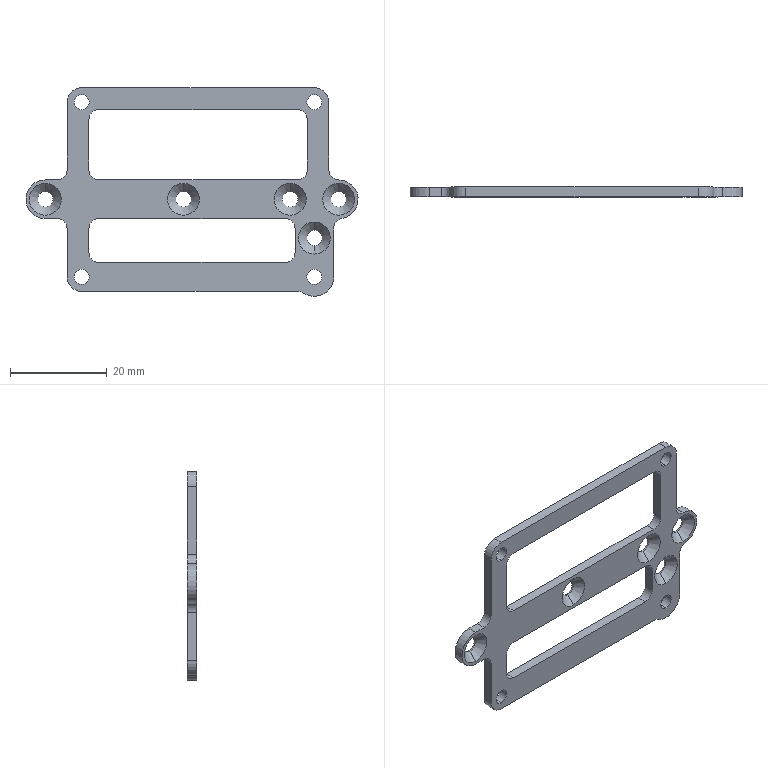Part | SolidWorks | features Extrusion 1, Fillet 1, HoleWzd 1 | 1 solid | 66 faces | box 68.5 x 2 x 43 mm | volume 2475 mm3 | cylinder 38 | plane 18 | cone 10 | commonest cylinder face diameters 4 x13 3.2 x10 3.1 x8 8 x4 6 x3